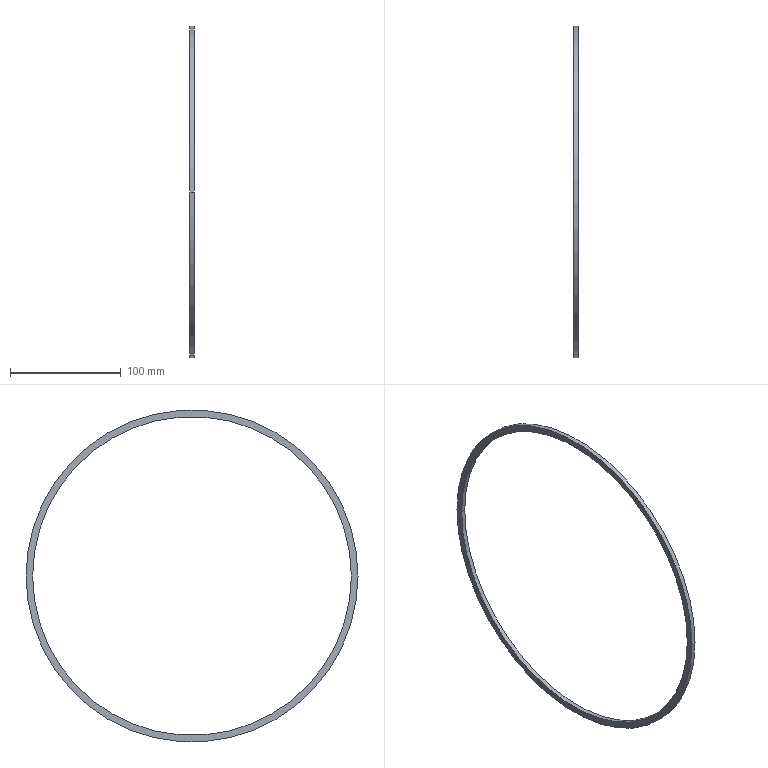Part | SolidWorks | features BaseBody 1 | 1 solid | 6 faces | box 4.288 x 300.004 x 300 mm | volume 22167 mm3 | cylinder 4 | plane 2 | commonest cylinder face diameters 288 x2 300 x2
STEP:
#1=CARTESIAN_POINT('',(299.027,315.923,106.919));
#2=VERTEX_POINT('',#1);
#3=CARTESIAN_POINT('',(298.739,615.923,106.919));
#4=VERTEX_POINT('',#3);
#5=CARTESIAN_POINT('',(298.883,465.923,106.919));
#6=DIRECTION('',(1.,0.0009599,0.));
#7=DIRECTION('',(0.0009599,-1.,0.));
#8=AXIS2_PLACEMENT_3D('',#5,#6,#7);
#9=CIRCLE('',#8,150.);
#10=EDGE_CURVE('',#2,#4,#9,.T.);
#11=ORIENTED_EDGE('',*,*,#10,.F.);
#12=CARTESIAN_POINT('',(295.027,315.919,106.919));
#13=VERTEX_POINT('',#12);
#14=CARTESIAN_POINT('',(299.027,315.923,106.919));
#15=DIRECTION('',(-1.,-0.0009599,0.));
#16=VECTOR('',#15,1000.);
#17=LINE('',#14,#16);
#18=EDGE_CURVE('',#2,#13,#17,.T.);
#19=ORIENTED_EDGE('',*,*,#18,.T.);
#20=CARTESIAN_POINT('',(294.739,615.919,106.919));
#21=VERTEX_POINT('',#20);
#22=CARTESIAN_POINT('',(294.883,465.919,106.919));
#23=DIRECTION('',(-1.,-0.0009599,0.));
#24=DIRECTION('',(-0.0009599,1.,0.));
#25=AXIS2_PLACEMENT_3D('',#22,#23,#24);
#26=CIRCLE('',#25,150.);
#27=EDGE_CURVE('',#21,#13,#26,.T.);
#28=ORIENTED_EDGE('',*,*,#27,.F.);
#29=CARTESIAN_POINT('',(298.739,615.923,106.919));
#30=DIRECTION('',(-1.,-0.0009599,0.));
#31=VECTOR('',#30,1000.);
#32=LINE('',#29,#31);
#33=EDGE_CURVE('',#4,#21,#32,.T.);
#34=ORIENTED_EDGE('',*,*,#33,.F.);
#35=EDGE_LOOP('',(#11,#19,#28,#34));
#36=FACE_OUTER_BOUND('',#35,.T.);
#37=CARTESIAN_POINT('',(298.883,465.923,106.919));
#38=DIRECTION('',(-1.,-0.0009599,0.));
#39=DIRECTION('',(-0.0009599,1.,0.));
#40=AXIS2_PLACEMENT_3D('',#37,#38,#39);
#41=CYLINDRICAL_SURFACE('',#40,150.);
#42=ADVANCED_FACE('',(#36),#41,.T.);
#43=CARTESIAN_POINT('',(299.021,321.923,106.919));
#44=VERTEX_POINT('',#43);
#45=CARTESIAN_POINT('',(298.744,609.923,106.919));
#46=VERTEX_POINT('',#45);
#47=CARTESIAN_POINT('',(298.883,465.923,106.919));
#48=DIRECTION('',(-1.,-0.0009599,0.));
#49=DIRECTION('',(0.0009599,-1.,0.));
#50=AXIS2_PLACEMENT_3D('',#47,#48,#49);
#51=CIRCLE('',#50,144.);
#52=EDGE_CURVE('',#44,#46,#51,.T.);
#53=ORIENTED_EDGE('',*,*,#52,.F.);
#54=CARTESIAN_POINT('',(295.021,321.919,106.919));
#55=VERTEX_POINT('',#54);
#56=CARTESIAN_POINT('',(299.021,321.923,106.919));
#57=DIRECTION('',(-1.,-0.0009599,0.));
#58=VECTOR('',#57,1000.);
#59=LINE('',#56,#58);
#60=EDGE_CURVE('',#44,#55,#59,.T.);
#61=ORIENTED_EDGE('',*,*,#60,.T.);
#62=CARTESIAN_POINT('',(294.744,609.919,106.919));
#63=VERTEX_POINT('',#62);
#64=CARTESIAN_POINT('',(294.883,465.919,106.919));
#65=DIRECTION('',(1.,0.0009599,0.));
#66=DIRECTION('',(0.0009599,-1.,0.));
#67=AXIS2_PLACEMENT_3D('',#64,#65,#66);
#68=CIRCLE('',#67,144.);
#69=EDGE_CURVE('',#63,#55,#68,.T.);
#70=ORIENTED_EDGE('',*,*,#69,.F.);
#71=CARTESIAN_POINT('',(298.744,609.923,106.919));
#72=DIRECTION('',(-1.,-0.0009599,0.));
#73=VECTOR('',#72,1000.);
#74=LINE('',#71,#73);
#75=EDGE_CURVE('',#46,#63,#74,.T.);
#76=ORIENTED_EDGE('',*,*,#75,.F.);
#77=EDGE_LOOP('',(#53,#61,#70,#76));
#78=FACE_OUTER_BOUND('',#77,.T.);
#79=CARTESIAN_POINT('',(298.883,465.923,106.919));
#80=DIRECTION('',(-1.,-0.0009599,0.));
#81=DIRECTION('',(-0.0009599,1.,0.));
#82=AXIS2_PLACEMENT_3D('',#79,#80,#81);
#83=CYLINDRICAL_SURFACE('',#82,144.);
#84=ADVANCED_FACE('',(#78),#83,.F.);
#85=ORIENTED_EDGE('',*,*,#69,.T.);
#86=CARTESIAN_POINT('',(294.883,465.919,106.919));
#87=DIRECTION('',(1.,0.0009599,0.));
#88=DIRECTION('',(0.0009599,-1.,0.));
#89=AXIS2_PLACEMENT_3D('',#86,#87,#88);
#90=CIRCLE('',#89,144.);
#91=EDGE_CURVE('',#55,#63,#90,.T.);
#92=ORIENTED_EDGE('',*,*,#91,.T.);
#93=EDGE_LOOP('',(#85,#92));
#94=FACE_BOUND('',#93,.T.);
#95=ORIENTED_EDGE('',*,*,#27,.T.);
#96=CARTESIAN_POINT('',(294.883,465.919,106.919));
#97=DIRECTION('',(-1.,-0.0009599,0.));
#98=DIRECTION('',(-0.0009599,1.,0.));
#99=AXIS2_PLACEMENT_3D('',#96,#97,#98);
#100=CIRCLE('',#99,150.);
#101=EDGE_CURVE('',#13,#21,#100,.T.);
#102=ORIENTED_EDGE('',*,*,#101,.T.);
#103=EDGE_LOOP('',(#95,#102));
#104=FACE_OUTER_BOUND('',#103,.T.);
#105=CARTESIAN_POINT('',(294.883,465.919,106.919));
#106=DIRECTION('',(-1.,-0.0009599,0.));
#107=DIRECTION('',(-0.0009599,1.,0.));
#108=AXIS2_PLACEMENT_3D('',#105,#106,#107);
#109=PLANE('',#108);
#110=ADVANCED_FACE('',(#94,#104),#109,.T.);
#111=ORIENTED_EDGE('',*,*,#60,.F.);
#112=CARTESIAN_POINT('',(298.883,465.923,106.919));
#113=DIRECTION('',(-1.,-0.0009599,0.));
#114=DIRECTION('',(0.0009599,-1.,0.));
#115=AXIS2_PLACEMENT_3D('',#112,#113,#114);
#116=CIRCLE('',#115,144.);
#117=EDGE_CURVE('',#46,#44,#116,.T.);
#118=ORIENTED_EDGE('',*,*,#117,.F.);
#119=ORIENTED_EDGE('',*,*,#75,.T.);
#120=ORIENTED_EDGE('',*,*,#91,.F.);
#121=EDGE_LOOP('',(#111,#118,#119,#120));
#122=FACE_OUTER_BOUND('',#121,.T.);
#123=CARTESIAN_POINT('',(298.883,465.923,106.919));
#124=DIRECTION('',(-1.,-0.0009599,0.));
#125=DIRECTION('',(-0.0009599,1.,0.));
#126=AXIS2_PLACEMENT_3D('',#123,#124,#125);
#127=CYLINDRICAL_SURFACE('',#126,144.);
#128=ADVANCED_FACE('',(#122),#127,.F.);
#129=ORIENTED_EDGE('',*,*,#117,.T.);
#130=ORIENTED_EDGE('',*,*,#52,.T.);
#131=EDGE_LOOP('',(#129,#130));
#132=FACE_BOUND('',#131,.T.);
#133=CARTESIAN_POINT('',(298.883,465.923,106.919));
#134=DIRECTION('',(1.,0.0009599,0.));
#135=DIRECTION('',(0.0009599,-1.,0.));
#136=AXIS2_PLACEMENT_3D('',#133,#134,#135);
#137=CIRCLE('',#136,150.);
#138=EDGE_CURVE('',#4,#2,#137,.T.);
#139=ORIENTED_EDGE('',*,*,#138,.T.);
#140=ORIENTED_EDGE('',*,*,#10,.T.);
#141=EDGE_LOOP('',(#139,#140));
#142=FACE_OUTER_BOUND('',#141,.T.);
#143=CARTESIAN_POINT('',(298.883,465.923,106.919));
#144=DIRECTION('',(-1.,-0.0009599,0.));
#145=DIRECTION('',(-0.0009599,1.,0.));
#146=AXIS2_PLACEMENT_3D('',#143,#144,#145);
#147=PLANE('',#146);
#148=ADVANCED_FACE('',(#132,#142),#147,.F.);
#149=ORIENTED_EDGE('',*,*,#18,.F.);
#150=ORIENTED_EDGE('',*,*,#138,.F.);
#151=ORIENTED_EDGE('',*,*,#33,.T.);
#152=ORIENTED_EDGE('',*,*,#101,.F.);
#153=EDGE_LOOP('',(#149,#150,#151,#152));
#154=FACE_OUTER_BOUND('',#153,.T.);
#155=CARTESIAN_POINT('',(298.883,465.923,106.919));
#156=DIRECTION('',(-1.,-0.0009599,0.));
#157=DIRECTION('',(-0.0009599,1.,0.));
#158=AXIS2_PLACEMENT_3D('',#155,#156,#157);
#159=CYLINDRICAL_SURFACE('',#158,150.);
#160=ADVANCED_FACE('',(#154),#159,.T.);
#161=CLOSED_SHELL('',(#42,#84,#110,#128,#148,#160));
#162=MANIFOLD_SOLID_BREP('',#161);
#163=CARTESIAN_POINT('',(0.,0.,0.));
#164=DIRECTION('',(0.,0.,1.));
#165=DIRECTION('',(1.,0.,0.));
#166=AXIS2_PLACEMENT_3D('',#163,#164,#165);
#167=(LENGTH_UNIT()NAMED_UNIT(*)SI_UNIT(.MILLI.,.METRE.));
#168=UNCERTAINTY_MEASURE_WITH_UNIT(LENGTH_MEASURE(0.00001),#167,'','');
#169=(NAMED_UNIT(*)PLANE_ANGLE_UNIT()SI_UNIT($,.RADIAN.));
#170=(NAMED_UNIT(*)SI_UNIT($,.STERADIAN.)SOLID_ANGLE_UNIT());
#171=(GEOMETRIC_REPRESENTATION_CONTEXT(3)GLOBAL_UNCERTAINTY_ASSIGNED_CONTEXT((#168))GLOBAL_UNIT_ASSIGNED_CONTEXT((#167,#169,#170))REPRESENTATION_CONTEXT('',''));
#172=ADVANCED_BREP_SHAPE_REPRESENTATION('',(#162,#166),#171);